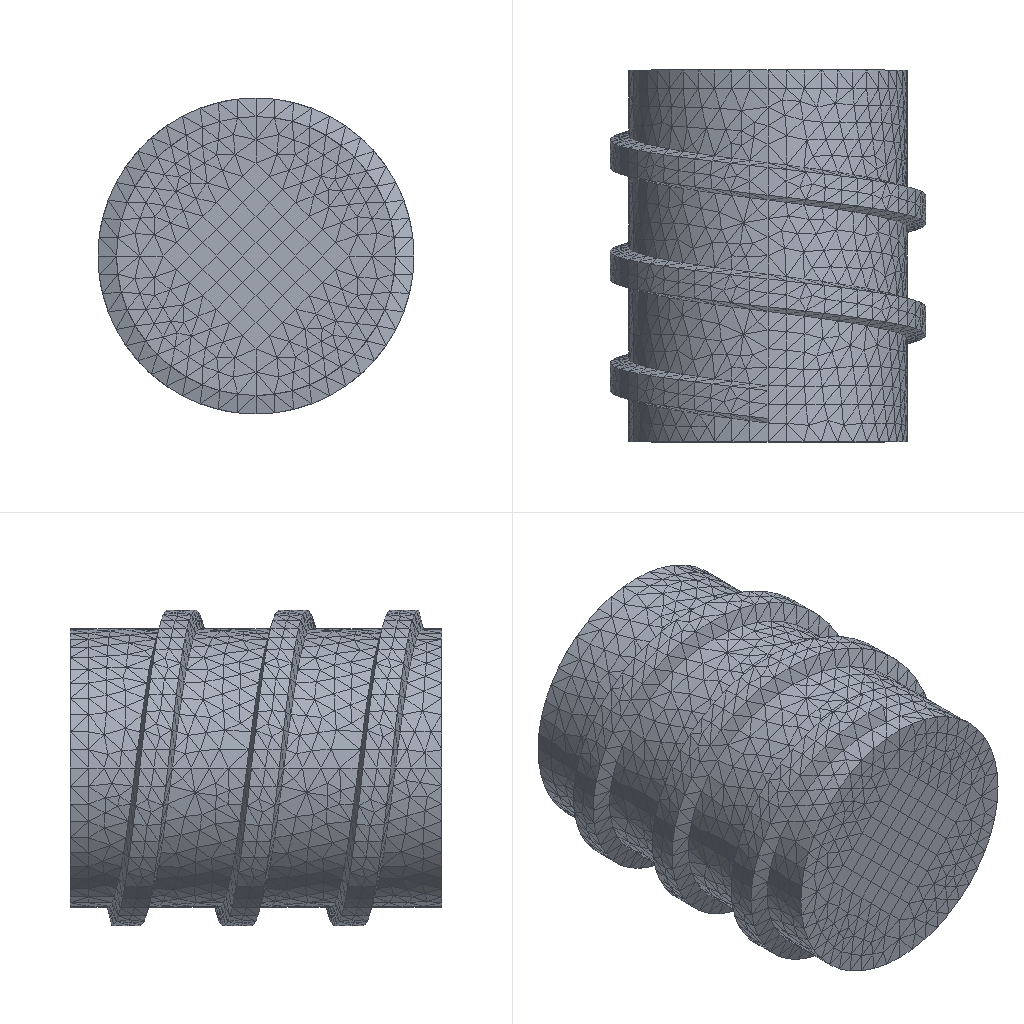Simulation study | abaqus
Set-up summary:
category,name,step,type,value,unit,region
solver,abaqus
solver,version,,,Abaqus/Standard 2020
units,not stated in the deck,,not stated
analysis,deck,,static,static
load_step,Step-1,Step-1,static
load_step,requested,,,1
mesh,nodes,,,6115
mesh,elements,,,23787
element_type,C3D4,,solid,22797
element_type,R3D4,,rigid,10
element_type,C3D8R,,solid,980
load,load commands in deck,,count,1
bc,support commands in deck,,count,17
material,MATERIAL-1,,in results
check,setup vs results,,match,"per instance, exact: element labels, types and connectivity; labels of the nodes the elements use; coordinates of those nodes at SINGLE_PRECISION in 2 of 2 instance(s)"
Abaqus input file, long lists of numbers shortened:
*Heading
** Job name: forth Model name: Model-3
** Generated by: Abaqus/CAE 2020
*Preprint, echo=NO, model=NO, history=NO, contact=NO
**
** PARTS
**
*Part, name=Part-2
*Node
      1,          55.,           0.,           0.
      2,          60.,           0.,           0.
** (20 more lines like these left out)
*Element, type=R3D4
 1,  1,  2,  4,  3
 2,  3,  4,  6,  5
** (8 more lines like these left out)
*Node
     23,   49.332,   34.153,           0.
*Nset, nset=Part-2-RefPt_, internal
23,
*Elset, elset=Part-2, generate
  1,  10,   1
*End Part
**
*Part, name=gangbang3
*Node
      1,         -20.,          80.,           0.
      2,           0.,          80.,          20.
** (6090 more lines like these left out)
*Element, type=C3D8R
  1,   10,  206, 3093,  117,    1,   69,  879,   92
  2,  206,  205, 3094, 3093,   69,   70,  880,  879
** (978 more lines like these left out)
*Element, type=C3D4
 981, 3777,  249, 1906, 1893
 982, 3777,  262,  250,   19
** (22795 more lines like these left out)
*Nset, nset=Set-17, generate
    1,  6092,     1
*Elset, elset=Set-17, generate
     1,  23777,      1
** Section: Section-1
*Solid Section, elset=Set-17, material=Material-1
,
*End Part
**
**
** ASSEMBLY
**
*Assembly, name=Assembly
**
*Instance, name=Part-2-1, part=Part-2
-25.058, 30., -14.753
-25.058, 30., -14.753, -24.077, 29.862, -14.614, 82.607
*End Instance
**
*Instance, name=gangbang3-1, part=gangbang3
*End Instance
**
*Node
      1,           0.,          90., -1.71574348e-15
*Nset, nset=Set-5, instance=gangbang3-1
    5,    6,    7,    8,   25,   26,   39,   57,   93,   94,   95,   96,   97,   98,   99,  100
  101,  102,  103,  104,  105,  106,  107,  108,  109,  110,  111,  112,  113,  114,  115,  116
** (12 more lines like these left out)
*Elset, elset=Set-5, instance=gangbang3-1
   932,   933,   934,   935,   936,   937,   938,   939,   940,   941,   942,   943,   944,   945,   946,   947
   948,   949,   950,   951,   952,   953,   954,   955,   956,   957,   958,   959,   960,   961,   962,   963
** (19 more lines like these left out)
*Nset, nset=Set-6
 1,
*Nset, nset=Set-7, instance=Part-2-1, generate
  1,  22,   1
*Nset, nset=Set-7, instance=gangbang3-1, generate
    1,  6092,     1
*Nset, nset=Set-7
 1,
*Elset, elset=Set-7, instance=Part-2-1, generate
  1,  10,   1
*Elset, elset=Set-7, instance=gangbang3-1, generate
     1,  23777,      1
*Nset, nset=Set-8, instance=Part-2-1, generate
  1,  22,   1
*Nset, nset=Set-8, instance=gangbang3-1, generate
    1,  6092,     1
*Nset, nset=Set-8
 1,
*Elset, elset=Set-8, instance=Part-2-1, generate
  1,  10,   1
*Elset, elset=Set-8, instance=gangbang3-1, generate
     1,  23777,      1
*Nset, nset=Set-9, instance=gangbang3-1
   13,   14,   15,   16,   17,   18,   19,   20,   23,   24,   27,   28,   29,   30,   31,   32
   33,   34,   35,   36,   37,   38,   41,   42,   43,   44,   45,   46,   47,   48,   49,   50
** (54 more lines like these left out)
*Elset, elset=Set-9, instance=gangbang3-1
   981,   982,   983,   984,   985,   986,   987,   988,   989,   990,   991,   992,   993,   994,   995,   996
   997,   998,   999,  1000,  1001,  1002,  1003,  1004,  1005,  1006,  1007,  1008,  1009,  1010,  1011,  1012
** (131 more lines like these left out)
*Nset, nset=m_Set-3
 1,
*Nset, nset=m_Set-4
 1,
*Nset, nset=_PickedSet6, internal, instance=gangbang3-1, generate
    1,  6092,     1
*Elset, elset=_PickedSet6, internal, instance=gangbang3-1, generate
     1,  23777,      1
*Nset, nset=_PickedSet7, internal, instance=Part-2-1, generate
  1,  22,   1
*Elset, elset=_PickedSet7, internal, instance=Part-2-1, generate
  1,  10,   1
*Elset, elset=_s_Surf-1_S2, internal, instance=gangbang3-1
     1,     2,     3,     4,     5,     6,     7,     8,     9,    10,    11,    12,    13,    14,    15,    16
    17,    18,    19,    20,    21,    22,    23,    24,    25,    26,    27,    28,    29,    30,    31,    32
** (4 more lines like these left out)
*Elset, elset=_s_Surf-1_S3, internal, instance=gangbang3-1
 22568, 22570, 22574, 22580, 22583, 22588, 22592, 22601, 22612, 22613, 22616, 22623, 22631, 22636, 22637, 22642
 22678, 22693, 22695, 22709, 22727, 22731, 22735, 22762, 22774, 22781, 22791, 22809, 22818, 22840, 22848, 22865
** (10 more lines like these left out)
*Elset, elset=_s_Surf-1_S4, internal, instance=gangbang3-1
 22573, 22611, 22648, 22651, 22654, 22656, 22677, 22742, 22771, 22847, 22910, 22976, 23019, 23054, 23073, 23109
 23170, 23253, 23320, 23372, 23381, 23432, 23454, 23466, 23538, 23631, 23647, 23651, 23676, 23704, 23744, 23751
** (1 more lines like these left out)
*Elset, elset=_s_Surf-1_S1, internal, instance=gangbang3-1
 22614, 22657, 22662, 22665, 22667, 22702, 22714, 22719, 22729, 22753, 22763, 22807, 23024, 23031, 23077, 23123
 23124, 23149, 23165, 23183, 23185, 23319, 23660, 23738, 23746
*Surface, type=ELEMENT, name=s_Surf-1
_s_Surf-1_S2, S2
_s_Surf-1_S3, S3
_s_Surf-1_S4, S4
_s_Surf-1_S1, S1
*Elset, elset=_s_Surf-2_S2, internal, instance=gangbang3-1
     1,     2,     3,     4,     5,     6,     7,     8,     9,    10,    11,    12,    13,    14,    15,    16
    17,    18,    19,    20,    21,    22,    23,    24,    25,    26,    27,    28,    29,    30,    31,    32
** (5 more lines like these left out)
*Elset, elset=_s_Surf-2_S1, internal, instance=gangbang3-1
 22614, 22657, 22662, 22665, 22667, 22702, 22714, 22719, 22729, 22730, 22736, 22753, 22761, 22763, 22807, 22860
 23024, 23031, 23077, 23123, 23124, 23138, 23149, 23165, 23183, 23185, 23282, 23319, 23362, 23366, 23369, 23389
** (1 more lines like these left out)
*Elset, elset=_s_Surf-2_S3, internal, instance=gangbang3-1
 22568, 22570, 22574, 22580, 22583, 22585, 22588, 22592, 22595, 22596, 22601, 22610, 22612, 22613, 22616, 22623
 22631, 22636, 22637, 22642, 22657, 22678, 22693, 22695, 22709, 22727, 22731, 22735, 22738, 22742, 22746, 22762
** (14 more lines like these left out)
*Elset, elset=_s_Surf-2_S4, internal, instance=gangbang3-1
 22573, 22611, 22648, 22651, 22654, 22656, 22677, 22733, 22742, 22771, 22809, 22826, 22847, 22851, 22853, 22910
 22927, 22976, 23019, 23054, 23073, 23109, 23126, 23147, 23170, 23253, 23266, 23291, 23320, 23372, 23381, 23420
** (1 more lines like these left out)
*Surface, type=ELEMENT, name=s_Surf-2
_s_Surf-2_S2, S2
_s_Surf-2_S1, S1
_s_Surf-2_S4, S4
_s_Surf-2_S3, S3
*Rigid Body, ref node=Part-2-1.Part-2-RefPt_, elset=Part-2-1.Part-2
*Elset, elset=__T1_gangbang3-1_M_S6, internal, instance=gangbang3-1, generate
  50,  974,    7
*Surface, type=ELEMENT, name=_T1_gangbang3-1_M, internal
__T1_gangbang3-1_M_S6, S6
*Elset, elset=__T1_gangbang3-1_S_S4, internal, instance=gangbang3-1
 17445, 17672, 18823, 19251, 19427, 19590, 19731, 19941, 20367, 20382, 20663, 20783, 20833, 20857, 21051, 21141
 21344, 21407, 21631, 22337
*Elset, elset=__T1_gangbang3-1_S_S3, internal, instance=gangbang3-1
 17560, 17856, 18035, 18061, 19013, 19039, 19094, 19134, 19142, 19147, 19150, 19152, 19169, 19170, 19236, 19256
 19263, 19287, 19294, 19306, 19311, 19320, 19324, 19511, 19588, 19689, 19761, 19840, 19938, 19957, 19982, 20034
** (9 more lines like these left out)
*Elset, elset=__T1_gangbang3-1_S_S2, internal, instance=gangbang3-1
 19163, 20453, 20674, 20727, 20802, 21004, 21133, 21263, 21281, 21441
*Elset, elset=__T1_gangbang3-1_S_S1, internal, instance=gangbang3-1
 20146,
*Surface, type=ELEMENT, name=_T1_gangbang3-1_S, internal
__T1_gangbang3-1_S_S4, S4
__T1_gangbang3-1_S_S3, S3
__T1_gangbang3-1_S_S2, S2
__T1_gangbang3-1_S_S1, S1
*Tie, name=_T1_gangbang3-1, adjust=no
_T1_gangbang3-1_S, _T1_gangbang3-1_M
*Elset, elset=__T3_gangbang3-1_M_S4, internal, instance=gangbang3-1, generate
  56,  980,    7
*Surface, type=ELEMENT, name=_T3_gangbang3-1_M, internal
__T3_gangbang3-1_M_S4, S4
*Elset, elset=__T3_gangbang3-1_S_S3, internal, instance=gangbang3-1
 1606, 1616, 1621, 1628, 1655, 1706, 1909, 2766, 2804, 2816, 2854, 2864, 2875, 2895, 2906, 2909
 2917, 2932, 2956, 2975, 2976, 2981, 2987, 3044, 3048, 3051, 3101, 3130, 3144, 3149, 3160, 3164
** (10 more lines like these left out)
*Elset, elset=__T3_gangbang3-1_S_S4, internal, instance=gangbang3-1
 2041, 2651, 3695, 3799, 4226, 4426, 4632, 5816, 5835, 5890
*Elset, elset=__T3_gangbang3-1_S_S1, internal, instance=gangbang3-1
 2134, 5831
*Elset, elset=__T3_gangbang3-1_S_S2, internal, instance=gangbang3-1
 2809, 3045, 3337, 3404, 3548, 3637, 3649, 3803, 3825, 4284, 4944, 5833, 5887
*Surface, type=ELEMENT, name=_T3_gangbang3-1_S, internal
__T3_gangbang3-1_S_S3, S3
__T3_gangbang3-1_S_S4, S4
__T3_gangbang3-1_S_S2, S2
__T3_gangbang3-1_S_S1, S1
*Tie, name=_T3_gangbang3-1, adjust=no
_T3_gangbang3-1_S, _T3_gangbang3-1_M
*Elset, elset=__T5_gangbang3-1_M_S3, internal, instance=gangbang3-1
  50,  51,  52,  53,  54,  55,  56,  99, 100, 101, 102, 103, 104, 105, 148, 149
 150, 151, 152, 153, 154, 197, 198, 199, 200, 201, 202, 203, 246, 247, 248, 249
** (7 more lines like these left out)
*Surface, type=ELEMENT, name=_T5_gangbang3-1_M, internal
__T5_gangbang3-1_M_S3, S3
*Elset, elset=__T5_gangbang3-1_S_S3, internal, instance=gangbang3-1
 11963, 12054, 12188, 12340, 12394, 12533, 12625, 13532, 13539, 13545, 13553, 13558, 13569, 13575, 13605, 13611
 13626, 13671, 13676, 13682, 13686, 13694, 13771, 13772, 13781, 13789, 13798, 13813, 13829, 13831, 13839, 13845
** (10 more lines like these left out)
*Elset, elset=__T5_gangbang3-1_S_S1, internal, instance=gangbang3-1
 13320, 14883, 16287
*Elset, elset=__T5_gangbang3-1_S_S4, internal, instance=gangbang3-1
 13321, 13583, 13629, 13955, 14072, 14287, 14721, 15314, 15327, 15571, 15685, 15739, 16270, 16695
*Elset, elset=__T5_gangbang3-1_S_S2, internal, instance=gangbang3-1
 13775, 14049, 14081, 14119, 14235, 14298, 14487, 15518
*Surface, type=ELEMENT, name=_T5_gangbang3-1_S, internal
__T5_gangbang3-1_S_S3, S3
__T5_gangbang3-1_S_S1, S1
__T5_gangbang3-1_S_S4, S4
__T5_gangbang3-1_S_S2, S2
*Tie, name=_T5_gangbang3-1, adjust=no
_T5_gangbang3-1_S, _T5_gangbang3-1_M
*Elset, elset=__T7_gangbang3-1_M_S5, internal, instance=gangbang3-1
  92,  93,  94,  95,  96,  97,  98, 141, 142, 143, 144, 145, 146, 147, 190, 191
 192, 193, 194, 195, 196, 239, 240, 241, 242, 243, 244, 245, 288, 289, 290, 291
** (7 more lines like these left out)
*Surface, type=ELEMENT, name=_T7_gangbang3-1_M, internal
__T7_gangbang3-1_M_S5, S5
*Elset, elset=__T7_gangbang3-1_S_S4, internal, instance=gangbang3-1
  6530,  8084,  8105,  8644,  8861,  8901,  8984,  9674,  9957, 10133, 10318, 11108
*Elset, elset=__T7_gangbang3-1_S_S3, internal, instance=gangbang3-1
  8010,  8032,  8054,  8056,  8062,  8065,  8077,  8091,  8093,  8107,  8135,  8139,  8145,  8160,  8164,  8175
  8200,  8203,  8208,  8215,  8237,  8264,  8284,  8285,  8295,  8318,  8338,  8342,  8346,  8349,  8358,  8380
** (10 more lines like these left out)
*Elset, elset=__T7_gangbang3-1_S_S2, internal, instance=gangbang3-1
  8872,  8963,  9057, 10083, 10259
*Elset, elset=__T7_gangbang3-1_S_S1, internal, instance=gangbang3-1
 10552,
*Surface, type=ELEMENT, name=_T7_gangbang3-1_S, internal
__T7_gangbang3-1_S_S4, S4
__T7_gangbang3-1_S_S3, S3
__T7_gangbang3-1_S_S2, S2
__T7_gangbang3-1_S_S1, S1
*Tie, name=_T7_gangbang3-1, adjust=no
_T7_gangbang3-1_S, _T7_gangbang3-1_M
** Constraint: Constraint-1
*Coupling, constraint name=Constraint-1, ref node=m_Set-4, surface=s_Surf-2
*Kinematic
*Enrichment, name=Crack-1, type=PROPAGATION CRACK, elset=_PickedSet6
*End Assembly
*Amplitude, name=Amp-1, definition=SMOOTH STEP
             0.,              0.,              1.,              1.
**
** MATERIALS
**
*Material, name=Material-1
*Damage Initiation, criterion=MAXPS
780.,
*Damage Evolution, type=DISPLACEMENT
 0.034,
*Damage Stabilization
0.0001
*Density
 7.85e-09,
*Elastic
212000., 0.28
*Plastic
1135.,    0.
1235.,  0.08
1435., 0.098
*Initial Conditions, type=ENRICHMENT
gangbang3-1.137, 1,Crack-1, -0.7565, 3.163
gangbang3-1.137, 2,Crack-1, 3.581, 3.923
gangbang3-1.137, 3,Crack-1, 4.084, 0.01421
gangbang3-1.137, 4,Crack-1, 0.07147, -0.4503
gangbang3-1.195, 1,Crack-1, 3.581, 3.923
gangbang3-1.195, 2,Crack-1, -0.7565, 3.163
gangbang3-1.195, 3,Crack-1, -0.3293, 3.589
gangbang3-1.195, 4,Crack-1, 0.07147, -0.4503
gangbang3-1.195, 1,Crack-1, -0.3293, 3.589
gangbang3-1.195, 2,Crack-1, 0.07147, -0.4503
gangbang3-1.195, 3,Crack-1, -0.7565, 3.163
gangbang3-1.195, 4,Crack-1, -2.669, -0.4473
gangbang3-1.458, 1,Crack-1, -0.7565, 3.163
gangbang3-1.458, 2,Crack-1, -2.669, -0.4473
gangbang3-1.458, 3,Crack-1, 0.07147, -0.4503
gangbang3-1.458, 4,Crack-1, 1.395, -0.6359
gangbang3-1.481, 1,Crack-1, 0.07147, -0.4503
gangbang3-1.481, 2,Crack-1, -0.7565, 3.163
gangbang3-1.481, 3,Crack-1, 1.395, -0.6359
gangbang3-1.481, 4,Crack-1, 4.084, 0.01421
gangbang3-1.192, 1,Crack-1, -1.879, 2.365
gangbang3-1.192, 2,Crack-1, -0.7565, 3.163
gangbang3-1.192, 3,Crack-1, 1.395, -0.6359
gangbang3-1.192, 4,Crack-1, -2.669, -0.4473
gangbang3-1.312, 1,Crack-1, -0.3293, 3.589
gangbang3-1.312, 2,Crack-1, -2.669, -0.4473
gangbang3-1.312, 3,Crack-1, -2.886, -0.2752
gangbang3-1.312, 4,Crack-1, 0.07147, -0.4503
gangbang3-1.595, 1,Crack-1, -0.3293, 3.589
gangbang3-1.595, 2,Crack-1, 0.07147, -0.4503
gangbang3-1.595, 3,Crack-1, -2.886, -0.2752
gangbang3-1.595, 4,Crack-1, 1.711, -0.03946
gangbang3-1.562, 1,Crack-1, -2.351, 3.891
gangbang3-1.562, 2,Crack-1, -2.886, -0.2752
gangbang3-1.562, 3,Crack-1, 1.711, -0.03946
gangbang3-1.562, 4,Crack-1, -0.3293, 3.589
gangbang3-1.513, 1,Crack-1, -1.879, 2.365
gangbang3-1.513, 2,Crack-1, -2.669, -0.4473
gangbang3-1.513, 3,Crack-1, 1.395, -0.6359
gangbang3-1.513, 4,Crack-1, -2.087, -1.066
** (268 more lines like these left out)
**
** BOUNDARY CONDITIONS
**
** Name: BC-1 Type: 位移/转角
*Boundary
Set-5, 1, 1
Set-5, 2, 2
Set-5, 3, 3
Set-5, 4, 4
Set-5, 5, 5
Set-5, 6, 6
** ----------------------------------------------------------------
**
** STEP: Step-1
**
*Step, name=Step-1, nlgeom=YES, inc=10000
*Static, stabilize=0.0002, allsdtol=0.05, continue=NO
0.001, 1., 1e-10, 0.2
**
** BOUNDARY CONDITIONS
**
** Name: BC-2 Type: 位移/转角
*Boundary, amplitude=Amp-1
Set-6, 1, 1
Set-6, 2, 2, 1.4
Set-6, 3, 3
Set-6, 4, 4
Set-6, 5, 5
Set-6, 6, 6
** Name: BC-3 Type: 位移/转角
*Boundary
Set-9, 1, 1
Set-9, 3, 3
Set-9, 4, 4
Set-9, 5, 5
Set-9, 6, 6
**
** INTERACTIONS
**
** Interaction: Int-1
*Enrichment Activation, name=Crack-1, activate=ON
**
** CONTROLS
**
*Controls, reset
*Controls, parameters=time incrementation
, , , , , , , 20, , ,
**
** OUTPUT REQUESTS
**
*Restart, write, frequency=0
**
** FIELD OUTPUT: F-Output-1
**
*Output, field, frequency=5
*Node Output
CF, PHILSM, PSILSM, RF, U
*Element Output, directions=YES
DMICRT, LE, PE, PEEQ, PEMAG, S, STATUS
*Contact Output
CDISP, CSTRESS
**
** HISTORY OUTPUT: H-Output-1
**
*Output, history, variable=PRESELECT
*End Step
Results summary:
result,step,,partial,increments=319 time=0.2911/1.0
result,analysis,,,static
result,last_loadstep,,,1
result,primary field,,,U
result,reaction total,,FX,198.479,model units
result,reaction total,,FY,1220.545,model units
result,reaction total,,FZ,-326.318,model units